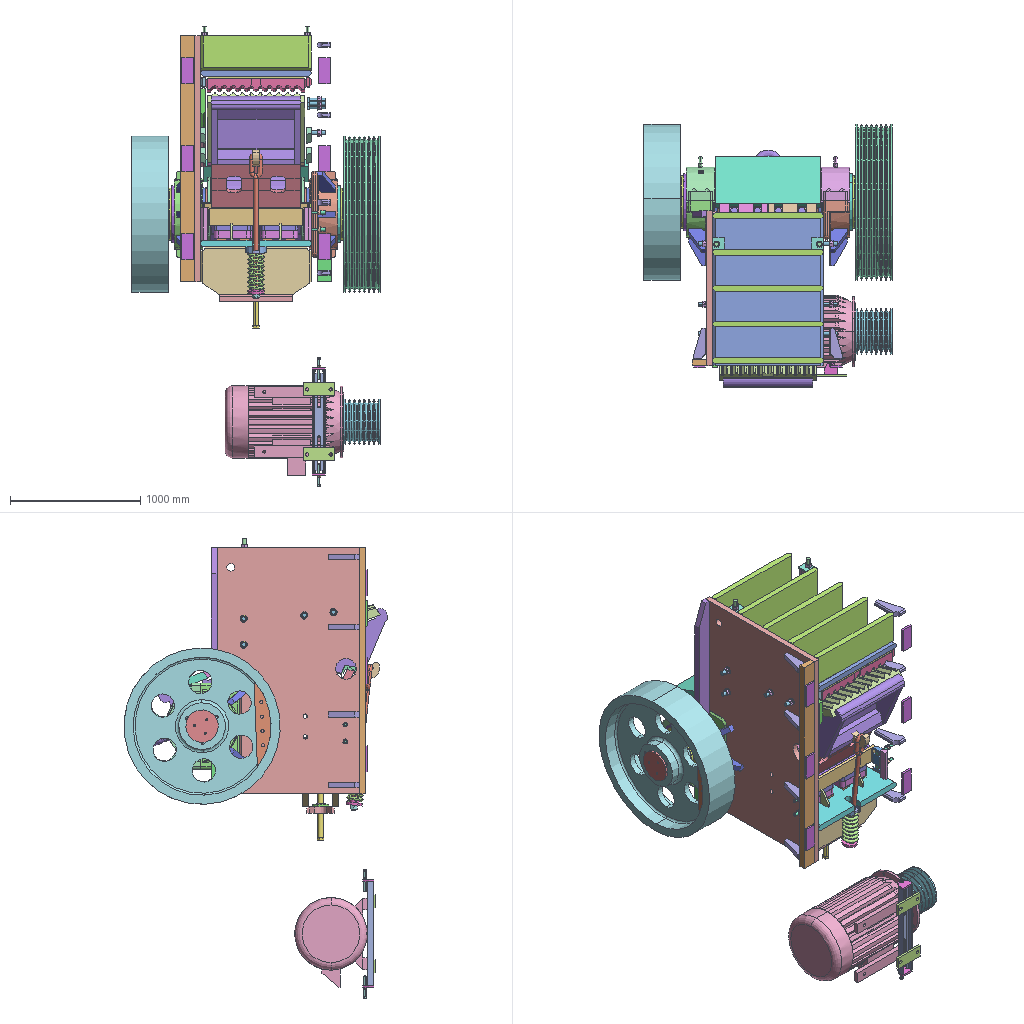Assembly | SolidWorks | 99 different items | 206 placed | box 1906 x 2026 x 3532 mm
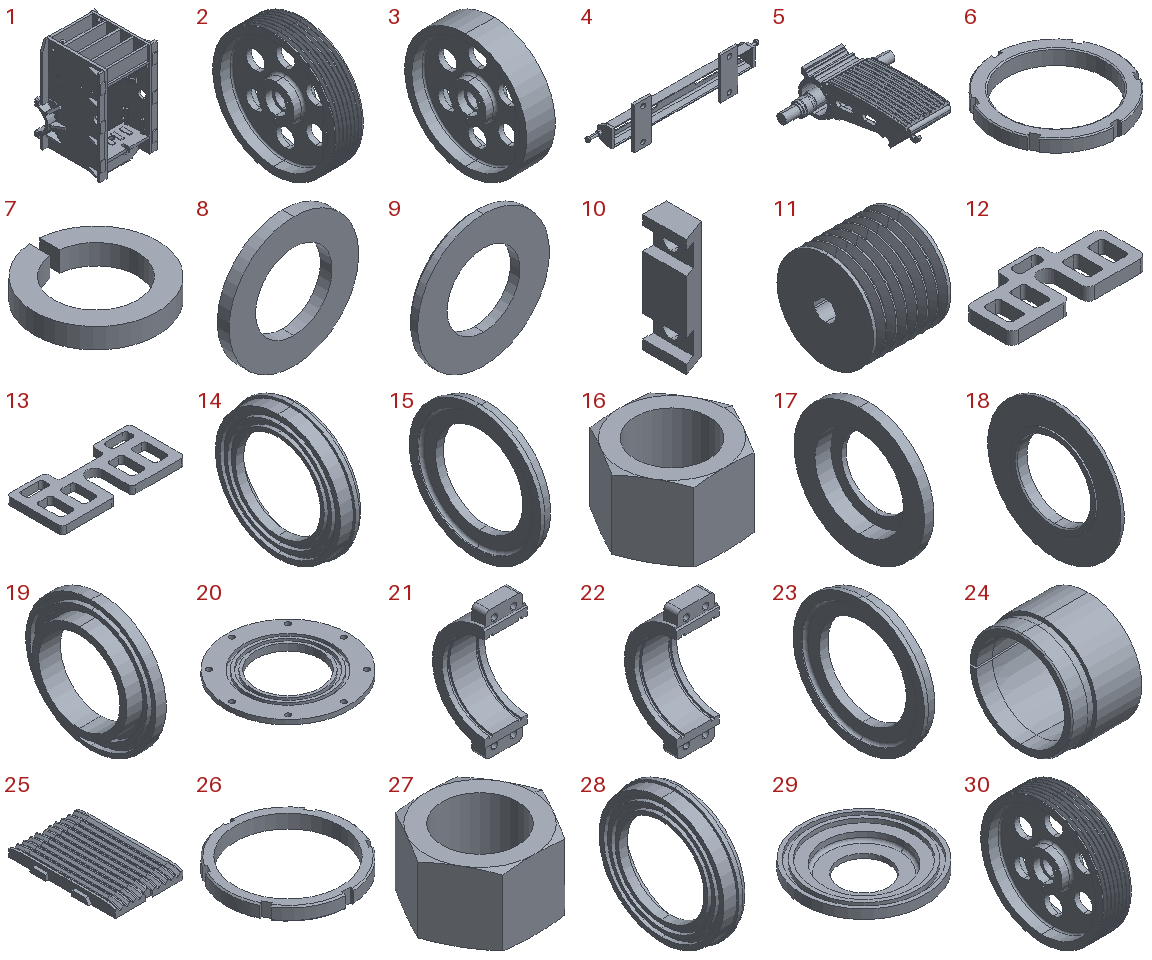Parts list (item | name | quantity | parent item | size | volume | features):
1 | (subassembly) | x1 | - | 1256 x 1280 x 2040 mm | 426098294 mm3 | features ReferencePattern 27, MirrorCompFeat 8, LocalCirPattern 2, LocalLPattern 1
2 | (subassembly) | x1 | - | 280 x 1200 x 1200 mm | 105552059 mm3 | features CompositeCurve 1
3 | (subassembly) | x1 | - | 280 x 1200 x 1200 mm | 122097534 mm3 | -
4 | (subassembly) | x1 | - | 984.816 x 100 x 240 mm | 1918082 mm3 | features ReferencePattern 4, MirrorCompFeat 3
5 | (subassembly) | x1 | - | 1846 x 2050 x 710.858 mm | 325009272 mm3 | features CompositeCurve 1
6 | - | x2 | - | 240 x 239.437 x 30 mm | 460595 mm3 | features Chamfer 3, CirPattern 1, Cut 1, Extrusion 1
7 | - | x4 | in 2 | 36.439 x 36.377 x 6 mm | 3321 mm3 | features Extrusion 1
8 | - | x4 | in 2 | 44 x 4 x 44 mm | 3958 mm3 | features Revolution 1
9 | - | x8 | - | 56 x 4 x 56 mm | 6746 mm3 | features Revolution 1
10 | - | x2 | - | 40 x 74.559 x 200 mm | 417359 mm3 | features ICE 2, Extrusion 1, MirrorPattern 1
11 | - | x1 | - | 280 x 349 x 349 mm | 15090387 mm3 | features ICE 1, LPattern 1, RevCut 1, Revolution 1
12 | - | x1 | - | 640 x 290 x 60 mm | 5683176 mm3 | features Fillet 2, Extrusion 1, ICE 1, MirrorPattern 1, PLine 1
13 | - | x1 | - | 640 x 290 x 40 mm | 4114262 mm3 | features Fillet 2, Extrusion 1, ICE 1, MirrorPattern 1, PLine 1
14 | - | x1 | - | 71 x 455 x 455 mm | 3180516 mm3 | features Revolution 1
15 | - | x1 | - | 41 x 455 x 455 mm | 2264387 mm3 | features Fillet 1, Revolution 1
16 | - | x2 | in 4 | 26.17 x 22.664 x 15.9 mm | 3864 mm3 | features Cut 2, Chamfer 1, Extrusion 1
17 | - | x2 | - | 63 x 404 x 404 mm | 2394632 mm3 | features Revolution 1
18 | - | x2 | - | 35 x 436 x 436 mm | 1356536 mm3 | features Chamfer 1, Revolution 1
19 | - | x2 | - | 64 x 384 x 384 mm | 2278534 mm3 | features Revolution 1
20 | - | x2 | - | 540 x 540 x 45 mm | 4136152 mm3 | features CirPattern 1, ICE 1, Revolution 1
21 | - | x1 | - | 218 x 352.5 x 660 mm | 9674169 mm3 | features ICE 5, 3DProfileFeature 1, Extrusion 1, Fillet 1, HoleWzd 1, MirrorPattern 1, RevCut 1, Revolution 1
22 | - | x1 | - | 218 x 352.5 x 660 mm | 9674169 mm3 | features ICE 5, 3DProfileFeature 1, Extrusion 1, Fillet 1, HoleWzd 1, MirrorPattern 1, RevCut 1, Revolution 1
23 | - | x1 | - | 44 x 455 x 455 mm | 2505652 mm3 | features Fillet 1, Revolution 1
24 | - | x2 | - | 151 x 239.983 x 240 mm | 1801757 mm3 | features Chamfer 1, ICE 1, Revolution 1
25 | - | x1 | - | 820 x 1170 x 110 mm | 61269041 mm3 | features Fillet 3, ICE 3, LPattern 3, MirrorPattern 2, Extrusion 1, SweepCut 1
26 | - | x2 | - | 270 x 269.399 x 30 mm | 439038 mm3 | features Chamfer 1, CirPattern 1, ICE 1, Revolution 1
27 | - | x4 | - | 39.55 x 34.251 x 22.3 mm | 12527 mm3 | features Cut 2, Chamfer 1, Extrusion 1
28 | - | x1 | - | 74 x 455 x 455 mm | 3257613 mm3 | features Revolution 1
29 | - | x2 | - | 404 x 404 x 56 mm | 2436851 mm3 | features Fillet 1, Revolution 1
30 | - | x1 | in 2 | 280 x 1200 x 1200 mm | 100101767 mm3 | features CirPattern 2, ICE 2, 3DProfileFeature 1, HoleWzd 1, LPattern 1, RevCut 1, Revolution 1
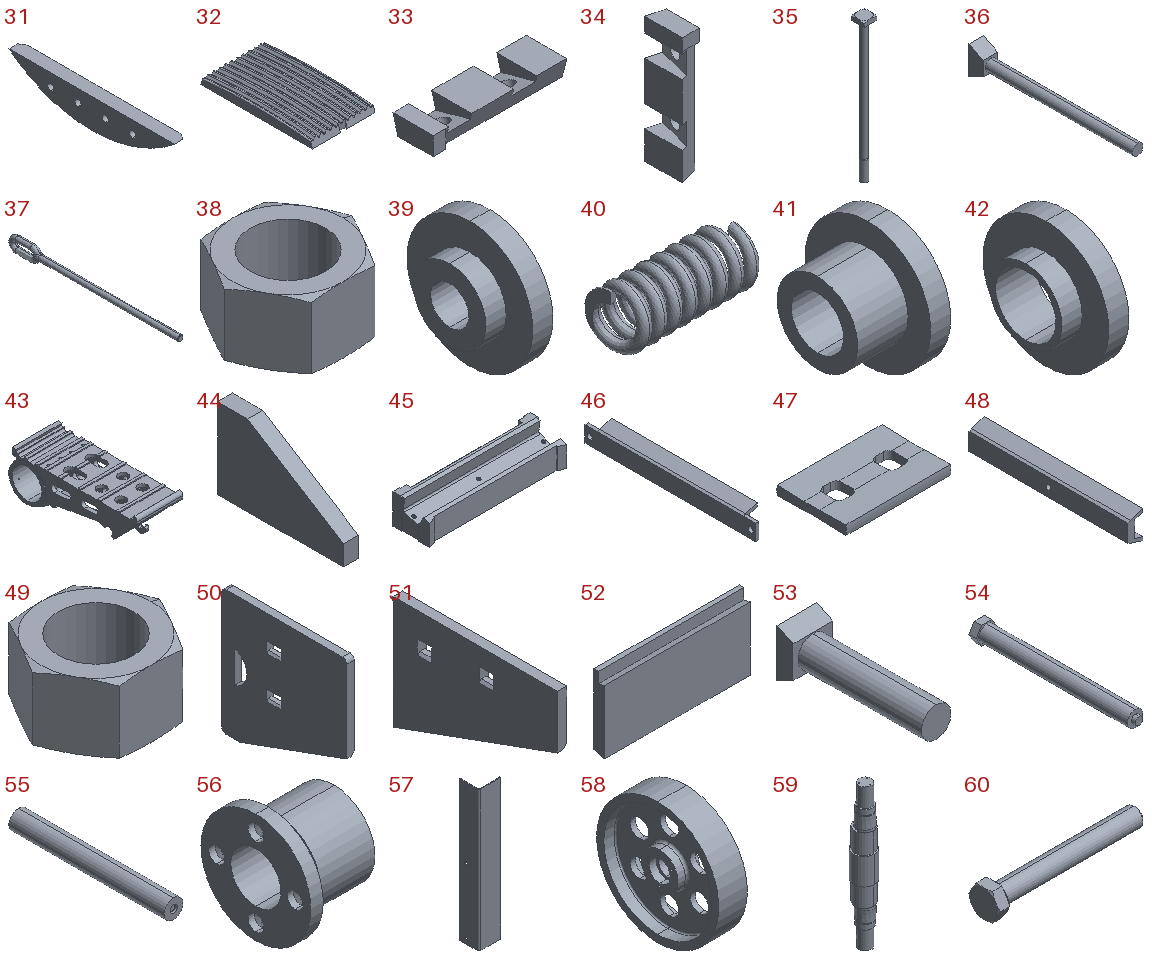31 | - | x4 | in 2, 3 | 50 x 666.801 x 118 mm | 2510197 mm3 | features Chamfer 1, Extrusion 1, ICE 1
32 | - | x1 | - | 750 x 1330 x 125.858 mm | 65171136 mm3 | features ICE 4, LPattern 2, MirrorPattern 2, Extrusion 1, Fillet 1, SweepCut 1
33 | - | x1 | - | 370 x 110.795 x 50 mm | 1371734 mm3 | features ICE 3, Extrusion 1, LPattern 1, RevCut 1
34 | - | x1 | - | 50 x 110.795 x 370 mm | 1371734 mm3 | features ICE 3, Extrusion 1, LPattern 1, RevCut 1
35 | - | x4 | - | 55 x 55 x 609 mm | 405608 mm3 | features Cut 1, Extrusion 1, Fillet 1, LPattern 1, RevCut 1, Revolution 1
36 | - | x2 | - | 40 x 450 x 80 mm | 385812 mm3 | features ICE 2, Extrusion 1
37 | - | x1 | - | 36 x 1131 x 102 mm | 1361962 mm3 | features Chamfer 1, Sweep 1
38 | - | x10 | - | 50.85 x 44.037 x 26.4 mm | 25591 mm3 | features Cut 2, Chamfer 1, Extrusion 1
39 | - | x1 | - | 40 x 125 x 125 mm | 281502 mm3 | features Revolution 1
40 | - | x1 | - | 280.817 x 125 x 125 mm | 1207735 mm3 | features Helix 1, ICE 1, Sweep 1
41 | - | x1 | - | 70 x 125 x 125 mm | 348104 mm3 | features Revolution 1
42 | - | x1 | - | 40 x 125 x 125 mm | 213770 mm3 | features Revolution 1
43 | - | x1 | - | 704 x 2050 x 634.865 mm | 188123623 mm3 | features ICE 12, MirrorPattern 5, 3DProfileFeature 4, HoleWzd 4, Fillet 2, CirPattern 1, Extrusion 1, Revolution 1
44 | - | x2 | - | 15 x 125 x 80 mm | 107250 mm3 | features Extrusion 1
45 | - | x1 | - | 800 x 215 x 175 mm | 15797212 mm3 | features ICE 5, 3DProfileFeature 2, HoleWzd 2, Extrusion 1, Fillet 1, MirrorPattern 1
46 | - | x1 | - | 65 x 800 x 120 mm | 2622134 mm3 | features ICE 2, Extrusion 1, MirrorPattern 1
47 | - | x1 | - | 680 x 450 x 60 mm | 14870230 mm3 | features Extrusion 1, ICE 1, MirrorPattern 1
48 | - | x1 | - | 65 x 682 x 120 mm | 2487309 mm3 | features Extrusion 1, ICE 1
49 | - | x1 | - | 60.79 x 52.646 x 31.9 mm | 43950 mm3 | features Cut 2, Chamfer 1, Extrusion 1
50 | - | x2 | - | 35 x 600 x 600 mm | 10412431 mm3 | features Chamfer 1, Extrusion 1, Fillet 1, ICE 1
51 | - | x2 | - | 35 x 600 x 413 mm | 6164844 mm3 | features ICE 2, Chamfer 1, Extrusion 1
52 | - | x1 | - | 800 x 60 x 400 mm | 17282858 mm3 | features Extrusion 1
53 | - | x8 | - | 40 x 140 x 48 mm | 113250 mm3 | features ICE 2, Extrusion 1
54 | - | x1 | - | 53 x 410 x 45.899 mm | 516586 mm3 | features ICE 1, Revolution 1
55 | - | x1 | - | 48 x 395 x 48 mm | 696230 mm3 | features 3DProfileFeature 1, HoleWzd 1, Revolution 1
56 | - | x1 | - | 50 x 70 x 70 mm | 75479 mm3 | features 3DProfileFeature 1, CirPattern 1, HoleWzd 1, Revolution 1
57 | - | x1 | - | 100 x 90 x 645 mm | 355061 mm3 | features FlatPattern 1, ICE 1, SMBaseFlange 1, SheetMetal 1
58 | - | x1 | in 3 | 280 x 1200 x 1200 mm | 117077142 mm3 | features CirPattern 2, ICE 2, 3DProfileFeature 1, HoleWzd 1, Revolution 1
59 | - | x1 | - | 270 x 270 x 1846 mm | 68110959 mm3 | features MirrorPattern 3, Revolution 2, 3DProfileFeature 1, CirPattern 1, HoleWzd 1, ICE 1
60 | - | x4 | in 2 | 200 x 41.569 x 36 mm | 100195 mm3 | features RevCut 4, Chamfer 1, Extrusion 1, Fillet 1, LPattern 1, Revolution 1
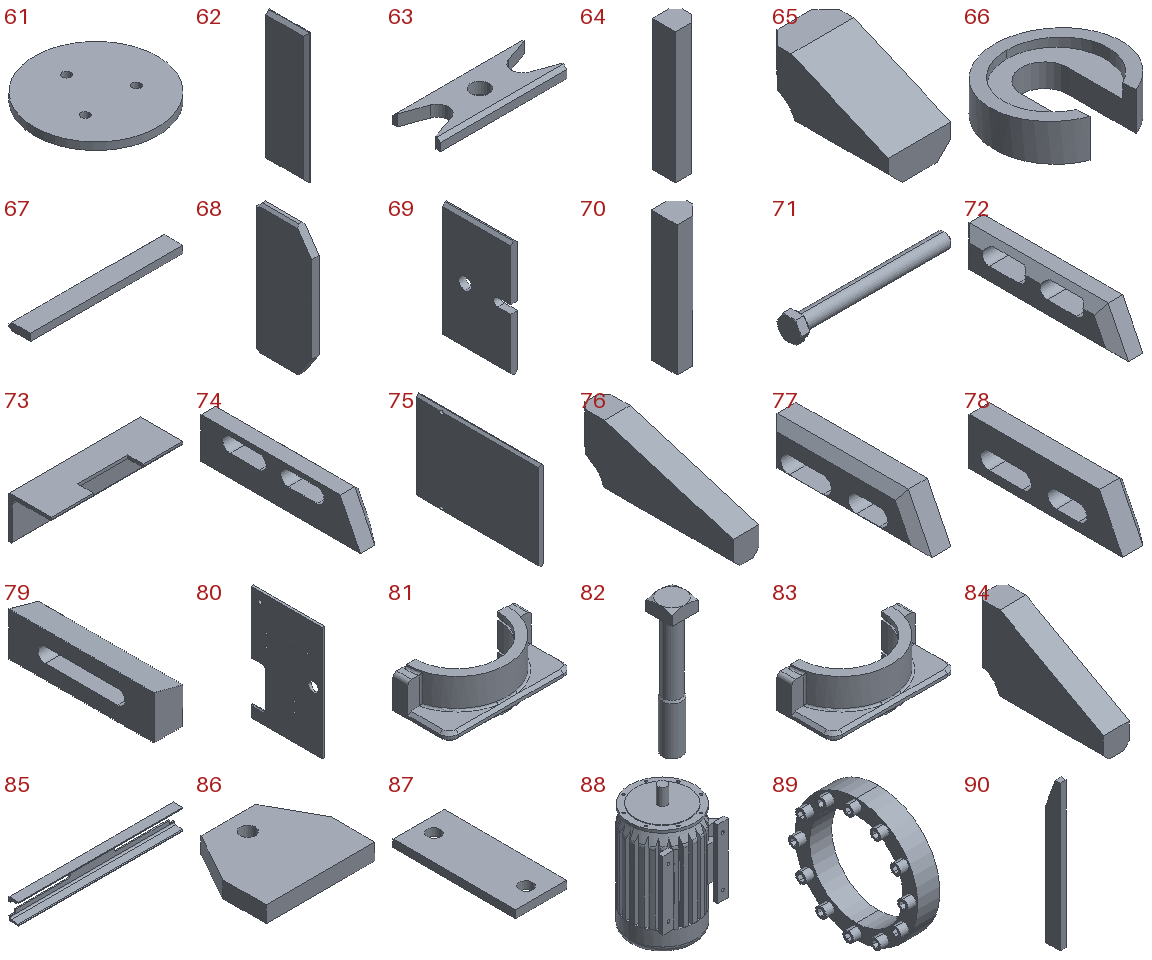61 | - | x2 | - | 250 x 250 x 15 mm | 726097 mm3 | features Extrusion 1
62 | - | x5 | in 1 | 45 x 265 x 850 mm | 9594917 mm3 | features Chamfer 1, Extrusion 1
63 | - | x1 | in 1 | 560 x 210 x 50 mm | 3864002 mm3 | features Chamfer 1, Extrusion 1
64 | - | x2 | in 1 | 50 x 50 x 280 mm | 637000 mm3 | features Chamfer 1, Extrusion 1
65 | - | x4 | in 1 | 45 x 90 x 50 mm | 124093 mm3 | features Chamfer 1, Extrusion 1
66 | - | x1 | in 1 | 160 x 154.162 x 49.592 mm | 478394 mm3 | features ICE 2, Revolution 1
67 | - | x2 | in 1 | 850 x 120 x 40 mm | 3888750 mm3 | features Chamfer 1, Extrusion 1
68 | - | x2 | in 1 | 50 x 370 x 850 mm | 14620496 mm3 | features Chamfer 1, Extrusion 1
69 | - | x1 | in 1 | 50 x 500 x 850 mm | 20176228 mm3 | features Chamfer 1, Extrusion 1
70 | - | x2 | in 1 | 50 x 50 x 250 mm | 525000 mm3 | features Chamfer 1, Extrusion 1
71 | - | x2 | in 4 | 170 x 27.713 x 24 mm | 37050 mm3 | features RevCut 4, Chamfer 1, Extrusion 1, Fillet 1, LPattern 1, Revolution 1
72 | - | x1 | in 1 | 40 x 275 x 70 mm | 515457 mm3 | features Chamfer 1, Extrusion 1
73 | - | x2 | in 1 | 250 x 80 x 80 mm | 217898 mm3 | features ICE 1, WeldMemberFeat 1, WeldmentFeature 1
74 | - | x1 | in 1 | 40 x 275 x 70 mm | 515457 mm3 | features Chamfer 1, Extrusion 1
75 | - | x1 | in 1 | 45 x 1170 x 850 mm | 43736327 mm3 | features Chamfer 1, Extrusion 1
76 | - | x8 | in 1 | 40 x 240 x 100 mm | 643693 mm3 | features Chamfer 1, Extrusion 1
77 | - | x1 | in 1 | 40 x 229 x 70 mm | 431150 mm3 | features Chamfer 1, Extrusion 1
78 | - | x1 | in 1 | 40 x 229 x 70 mm | 442689 mm3 | features Chamfer 1, Extrusion 1
79 | - | x4 | in 1 | 40 x 200 x 60 mm | 344562 mm3 | features Extrusion 1, ICE 1
80 | - | x2 | in 1 | 45 x 1185 x 1890 mm | 92721344 mm3 | features ICE 2, Chamfer 1, Extrusion 1, Fillet 1
81 | - | x1 | in 1 | 660 x 300 x 218 mm | 12799321 mm3 | features Fillet 3, ICE 2, MirrorPattern 2, 3DProfileFeature 1, Chamfer 1, Extrusion 1, HoleWzd 1, RevCut 1
82 | - | x4 | - | 32.173 x 32.173 x 165 mm | 73641 mm3 | features Cut 1, Extrusion 1, Fillet 1, LPattern 1, RevCut 1, Revolution 1
83 | - | x1 | in 1 | 660 x 300 x 218 mm | 12799321 mm3 | features Fillet 3, ICE 2, MirrorPattern 2, 3DProfileFeature 1, Chamfer 1, Extrusion 1, HoleWzd 1, RevCut 1
84 | - | x6 | in 1 | 45 x 220 x 140 mm | 896409 mm3 | features Chamfer 1, Extrusion 1
85 | - | x1 | in 4 | 800 x 48 x 100 mm | 931477 mm3 | features ICE 2, MirrorPattern 1, WeldMemberFeat 1, WeldmentFeature 1
86 | - | x2 | in 4 | 100 x 85 x 15 mm | 108316 mm3 | features 3DProfileFeature 1, Extrusion 1, HoleWzd 1
87 | - | x2 | in 4 | 100 x 240 x 15 mm | 344072 mm3 | features Extrusion 1, ICE 1
88 | - | x1 | - | 687.6 x 557.6 x 1050 mm | 215841244 mm3 | features Boss 7, Cut 3, CirPattern 2, Chamfer 1, Extrusion 1, Fillet 1
89 | - | x2 | - | 52 x 210 x 210 mm | 580630 mm3 | features CirPattern 1, ICE 1, Revolution 1
90 | - | x2 | in 1 | 45 x 110 x 1110 mm | 5170500 mm3 | features Extrusion 1
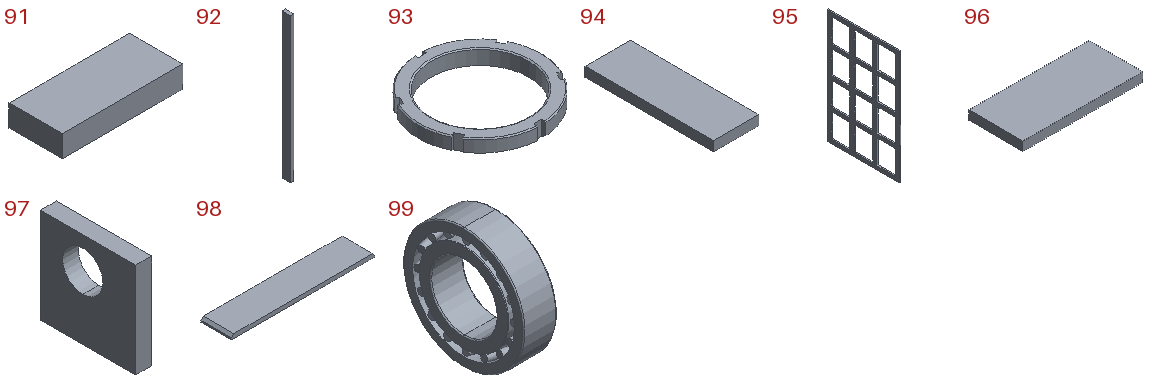91 | - | x2 | in 1 | 250 x 110 x 45 mm | 1237500 mm3 | features Extrusion 1
92 | - | x2 | in 1 | 45 x 110 x 1890 mm | 9355500 mm3 | features Extrusion 1
93 | - | x2 | - | 240 x 239.437 x 30 mm | 460595 mm3 | features Chamfer 3, CirPattern 1, Cut 1, Extrusion 1
94 | - | x4 | in 1 | 70 x 200 x 15 mm | 210000 mm3 | features Extrusion 1
95 | - | x1 | in 1 | 15 x 740 x 1170 mm | 4693500 mm3 | features Extrusion 1, ICE 1, MirrorPattern 1
96 | - | x6 | in 1 | 200 x 90 x 15 mm | 270000 mm3 | features Extrusion 1
97 | - | x2 | in 1 | 15 x 90 x 90 mm | 104488 mm3 | features Extrusion 1, ICE 1
98 | - | x1 | in 1 | 850 x 180 x 40 mm | 5852250 mm3 | features Chamfer 1, Extrusion 1
99 | - | x4 | - | 120 x 440 x 440 mm | 10049634 mm3 | features Revolution 3, CirPattern 1, MirrorPattern 1
Mates (type | each side: item.copy, entity, surface, feature):
In the top assembly
Coincident | 81.1 plane | assembly plane
Coincident | 1.1 plane | assembly plane | 2 times
Coincident | 95.1 face plane Boss-Extrude1 | 25.1 face plane Boss-Extrude1
Coincident | 25.1 plane | assembly plane
Coincident | 62.1 face plane Boss-Extrude1 | 25.1 face plane Boss-Extrude1
Coincident | 59.1 plane | assembly plane
Concentric | 81.1 face cylinder Boss-Extrude1 | 59.1 face cone Revolve2
Concentric | 59.1 face cylinder Revolve1 | 18.1 face cylinder Revolve1
Coincident | 59.1 face plane Revolve1 | 18.1 face plane Revolve1
Concentric | 59.1 face cylinder Revolve1 | 99.1 face cylinder Boss-Revolve1
Coincident | 18.1 face plane Revolve1 | 99.1 face plane Boss-Revolve1
Concentric | 59.1 face cylinder Revolve1 | 20.1 face cylinder Revolve1
Coincident | 99.1 face plane Base-Revolve1 | 20.1 face plane Revolve1
Concentric | 59.1 face cylinder Revolve1 | 19.1 face cylinder Revolve1
Coincident | 99.1 face plane Boss-Revolve1 | 19.1 face plane Revolve1
Coincident | 19.1 face plane Revolve1 | 17.1 face plane Revolve1
Concentric | 59.1 face cylinder Revolve2 | 17.1 face cylinder Revolve1
Concentric | 81.1 face cylinder Boss-Extrude1 | 23.1 face cylinder Revolve1
Coincident | 81.1 face plane Cut-Revolve1 | 23.1 face plane Revolve1
Concentric | 59.1 face cylinder Revolve2 | 24.1 face cylinder Revolve1
Coincident | 17.1 face plane Revolve1 | 24.1 face plane Revolve1
Concentric | 59.1 face cylinder Revolve2 | 28.1 face cylinder Revolve1
Coincident | 43.1 plane | assembly plane
Concentric | 59.1 face cylinder Revolve1 | 43.1 face cylinder Boss-Extrude1
Concentric | 20.1 face cylinder Cut-Extrude1 | 43.1 face cylinder CirPattern1
Coincident | 81.1 face plane Cut-Revolve1 | 28.1 face plane Revolve1
Concentric | 59.1 face cylinder Revolve2 | 99.2 face cylinder Base-Revolve1
Coincident | 23.1 face plane Revolve1 | 99.2 face plane Base-Revolve1
Concentric | 59.1 face cylinder Revolve2 | 26.1 face cylinder Revolve1
Coincident | 99.2 face plane Boss-Revolve1 | 26.1 face plane Revolve1
Concentric | 59.1 face cylinder Revolve2 | 93.1 face cylinder Base-Extrude
Concentric | 59.1 face cylinder Revolve2 | 6.1 face cylinder Base-Extrude
Coincident | 93.1 face plane Base-Extrude | 6.1 face plane Base-Extrude
Coincident | 26.1 face plane Revolve1 | 93.1 face plane Base-Extrude
Concentric | 59.1 face cylinder Revolve2 | 29.1 face cylinder Revolve1
Coincident | 59.1 face plane Revolve2 | 29.1 face plane Revolve1
Concentric | 81.1 face cylinder M30 Tapped Hole2 | 21.1 face cylinder Mirror1 | 2 times
Coincident | 81.1 face plane Boss-Extrude1 | 21.1 face plane Boss-Extrude2
Concentric | 59.1 face cylinder Revolve2 | 30.1 face cylinder Revolve1
Coincident | 29.1 face plane Revolve1 | 30.1 face plane Revolve1
Concentric | 59.1 face cylinder Revolve2 | 58.1 face cylinder Revolve1
Concentric | 59.1 face cylinder Mirror1 | 24.2 face cylinder Revolve1
Coincident | 17.2 face plane Revolve1 | 24.2 face plane Revolve1
Concentric | 59.1 face cylinder Mirror1 | 26.2 face cylinder Revolve1
Concentric | 59.1 face cylinder Mirror1 | 6.2 face cylinder Base-Extrude
Concentric | 59.1 face cylinder Mirror1 | 93.2 face cylinder Base-Extrude
Concentric | 59.1 face cylinder Mirror1 | 15.1 face cylinder Revolve1
Concentric | 59.1 face cylinder Mirror1 | 14.1 face cylinder Revolve1
Concentric | 59.1 face cylinder Mirror1 | 22.1 face cylinder Boss-Extrude2
Concentric | 83.1 face cylinder M30 Tapped Hole2 | 22.1 face cylinder Cut-Extrude1
Parallel | 80.1 face plane Boss-Extrude1 | 22.1 face plane Boss-Extrude3
Concentric | 59.1 face cylinder Mirror1 | 99.3 face cylinder Base-Revolve1
Coincident | 83.1 face plane Cut-Revolve1 | 14.1 face plane Revolve1
Coincident | 83.1 face plane Cut-Revolve1 | 15.1 face plane Revolve1
DistanceDim | 99.3 face plane Base-Revolve1 | 14.1 face plane Revolve1
Coincident | 26.2 face plane Revolve1 | 99.3 face plane Boss-Revolve1
Coincident | 93.2 face plane Base-Extrude | 6.2 face plane Base-Extrude
Coincident | 26.2 face plane Revolve1 | 93.2 face plane Base-Extrude
Concentric | 59.1 face cylinder Mirror1 | 29.2 face cylinder Revolve1
Coincident | 59.1 face plane Mirror1 | 29.2 face plane Revolve1
Coincident | 58.1 face plane Revolve1 | 29.2 face plane Revolve1
Concentric | 59.1 edge | 61.1 face cylinder Boss-Extrude1
Concentric | 59.1 edge | 89.1 face cylinder Revolve1
Coincident | 30.1 face plane Revolve1 | 89.1 face plane Revolve1
Coincident | 30.1 face plane Revolve1 | 61.1 face plane Boss-Extrude1
Concentric | 59.1 face cylinder M16 Tapped Hole1 | 61.1 face cylinder Boss-Extrude1
Coincident | 32.1 plane | assembly plane
Coincident | 43.1 face plane Boss-Extrude1 | 32.1 face plane Boss-Extrude1
Coincident | 43.1 face plane Boss-Extrude1 | 32.1 vertex
Coincident | 52.1 plane | assembly plane
Coincident | 43.1 face plane Boss-Extrude1 | 52.1 face plane Boss-Extrude1
Coincident | 43.1 face plane Boss-Extrude1 | 52.1 vertex
Concentric | 43.1 face cylinder Cut-Extrude2 | 34.1 face cylinder LPattern1
Concentric | 43.1 face cylinder Cut-Extrude2 | 34.1 face cylinder Cut-Revolve1
Coincident | 32.1 face plane Boss-Extrude1 | 34.1 vertex
Concentric | 43.1 face cylinder Cut-Extrude2 | 33.1 face cylinder LPattern1
Concentric | 43.1 face cylinder Cut-Extrude2 | 33.1 face cylinder Cut-Revolve1
Coincident | 32.1 face plane Boss-Extrude1 | 33.1 vertex
Concentric | 34.1 face cylinder Cut-Revolve1 | 35.1 face cylinder Boss-Revolve1
Coincident | 34.1 face plane Cut-Extrude2 | 35.1 vertex
Concentric | 33.1 face cylinder Cut-Revolve1 | 35.2 face cylinder Boss-Revolve1
Coincident | 33.1 face plane Cut-Extrude1 | 35.2 vertex
Coincident | 80.1 face plane Boss-Extrude1 | 51.1 face plane Boss-Extrude1
Parallel | 79.1 face plane Boss-Extrude1 | 51.1 face plane Boss-Extrude1
DistanceDim | 51.1 face plane Boss-Extrude1 | 80.1 face plane Boss-Extrude1
Tangent | 80.1 face cylinder Cut-Extrude1 | 51.1 face plane Cut-Extrude1
Coincident | 80.1 face plane Boss-Extrude1 | 50.1 face plane Boss-Extrude1
Parallel | 79.2 face plane Boss-Extrude1 | 50.1 face plane Boss-Extrude1
Tangent | 80.1 face cylinder Cut-Extrude1 | 50.1 face plane Cut-Extrude1
Coincident | 51.1 face plane Boss-Extrude1 | 50.1 face plane Boss-Extrude1
Concentric | 80.1 face cylinder Cut-Extrude1 | 53.1 face cylinder Boss-Extrude2
Concentric | 80.1 face cylinder Cut-Extrude1 | 53.2 face cylinder Boss-Extrude2
Concentric | 80.1 face cylinder Cut-Extrude1 | 53.3 face cylinder Boss-Extrude2
Concentric | 80.1 face cylinder Cut-Extrude1 | 53.4 face cylinder Boss-Extrude2
Coincident | 50.1 face plane Cut-Extrude1 | 53.2 edge
Coincident | 50.1 face plane Cut-Extrude1 | 53.1 edge
Coincident | 51.1 face plane Cut-Extrude1 | 53.3 edge
Coincident | 51.1 face plane Cut-Extrude2 | 53.4 edge
Concentric | 80.1 face cylinder Cut-Extrude1 | 9.1 face cylinder Base-Revolve
Coincident | 80.1 face plane Boss-Extrude1 | 9.1 face plane Base-Revolve
Concentric | 80.1 face cylinder Cut-Extrude1 | 9.2 face cylinder Base-Revolve
Coincident | 80.1 face plane Boss-Extrude1 | 9.2 face plane Base-Revolve
Concentric | 80.1 face cylinder Cut-Extrude1 | 9.3 face cylinder Base-Revolve
Coincident | 80.1 face plane Boss-Extrude1 | 9.3 face plane Base-Revolve
Concentric | 80.1 face cylinder Cut-Extrude1 | 9.4 face cylinder Base-Revolve
Coincident | 80.1 face plane Boss-Extrude1 | 9.4 face plane Base-Revolve
Concentric | 9.1 face cylinder Base-Revolve | 38.1 face cylinder Base-Extrude
Coincident | 9.1 face plane Base-Revolve | 38.1 face plane Base-Extrude
Concentric | 9.2 face cone Base-Revolve | 38.2 face cylinder Base-Extrude
Coincident | 9.2 face plane Base-Revolve | 38.2 face plane Base-Extrude
Concentric | 9.3 face cylinder Base-Revolve | 38.3 face cylinder Base-Extrude
Coincident | 9.3 face plane Base-Revolve | 38.3 face plane Base-Extrude
Concentric | 9.4 face cylinder Base-Revolve | 38.4 face cylinder Base-Extrude
Coincident | 9.4 face plane Base-Revolve | 38.4 face plane Base-Extrude
Symmetric | 43.1 face plane Boss-Extrude1 | 43.1 face plane Boss-Extrude1 | 48.1 plane
Concentric | 43.1 face cylinder M20 Tapped Hole1 | 48.1 face cylinder Cut-Extrude1
Coincident | 43.1 face plane Boss-Extrude1 | 48.1 face plane Boss-Extrude1
Coincident | 37.1 plane | assembly plane
Concentric | 43.1 edge | 37.1 select_type:24
DistanceDim | 32.1 vertex | 75.1 face plane Boss-Extrude1
PlanarAngleDim | 37.1 plane | 69.1 face plane Boss-Extrude1
Concentric | 66.1 face cylinder Revolve2 | 39.1 face cylinder Revolve1
Coincident | 66.1 face plane Revolve2 | 39.1 face plane Revolve1
Concentric | 39.1 face cylinder Revolve1 | 40.1 select_type:24
Coincident | 39.1 face plane Revolve1 | 40.1 face plane Cut-Extrude1
Concentric | 37.1 edge | 42.1 face cylinder Revolve1
Coincident | 40.1 vertex | 42.1 face plane Revolve1
Concentric | 42.1 edge | 49.1 edge
Coincident | 42.1 face plane Revolve1 | 49.1 face plane Base-Extrude
Coincident | 45.1 plane | assembly plane
Coincident | 46.1 plane | assembly plane
Symmetric | 45.1 face plane Boss-Extrude1 | 45.1 face plane Boss-Extrude1 | 46.1 plane
Coincident | 45.1 face plane Boss-Extrude1 | 46.1 face plane Boss-Extrude1
Concentric | 75.1 face cylinder Boss-Extrude1 | 36.1 face cylinder Boss-Extrude2
Coincident | 25.1 face plane Boss-Extrude2 | 36.1 edge
Concentric | 36.1 face cylinder Boss-Extrude2 | 38.5 face cylinder Base-Extrude
Coincident | 97.1 face plane Boss-Extrude1 | 38.5 face plane Base-Extrude
Coincident | 47.1 plane | assembly plane
Coincident | 70.1 face plane Boss-Extrude1 | 10.1 face plane Boss-Extrude1
DistanceDim | 10.1 face plane Boss-Extrude1 | 70.2 face plane Boss-Extrude1 | 2 times
Coincident | 45.1 face plane Cut-Extrude3 | 10.1 edge
Coincident | 12.1 plane | assembly plane
Coincident | 94.1 face plane Boss-Extrude1 | 12.1 face plane Boss-Extrude1
Coincident | 69.1 face plane Boss-Extrude1 | 44.1 face plane Boss-Extrude1
DistanceDim | assembly plane | 44.1 face plane Boss-Extrude1
Concentric | 10.1 face cylinder Cut-Extrude2 | 82.1 face cylinder Boss-Revolve1
Coincident | 10.1 face plane Mirror1 | 82.1 face plane Base-Extrude
Concentric | 10.1 face cylinder Cut-Extrude2 | 82.2 face cylinder Boss-Revolve1
Coincident | 10.1 face plane Cut-Extrude1 | 82.2 face plane Base-Extrude
Concentric | 82.1 face cone Cut-Revolve1 | 27.1 face cylinder Base-Extrude
Concentric | 82.2 face cone Cut-Revolve1 | 27.2 face cylinder Base-Extrude
Coincident | 80.1 face plane Boss-Extrude1 | 27.1 face plane Base-Extrude
Coincident | 80.1 face plane Boss-Extrude1 | 27.2 face plane Base-Extrude
Coincident | 94.2 face plane Boss-Extrude1 | 44.1 face plane Boss-Extrude1
Coincident | 44.1 face plane Boss-Extrude1 | 12.1 face plane Boss-Extrude1
Coincident | 13.1 plane | assembly plane
Coincident | 12.1 face plane Boss-Extrude1 | 13.1 face plane Boss-Extrude1
Coincident | 44.1 face plane Boss-Extrude1 | 13.1 face plane Boss-Extrude1
Coincident | 45.1 face plane Boss-Extrude1 | 13.1 face plane Boss-Extrude1
PlanarAngleDim | 47.1 face plane Boss-Extrude1 | 96.1 face plane Boss-Extrude1
Tangent | 46.1 face plane Boss-Extrude1 | 47.1 face cylinder Boss-Extrude1
Concentric | 63.1 edge | 41.1 face cylinder Revolve1
Coincident | 63.1 face plane Boss-Extrude1 | 41.1 face plane Revolve1
Coincident | 96.2 face plane Boss-Extrude1 | 88.1 face plane Extrude7
Concentric | 88.1 face cylinder Extrude1 | 11.1 face cylinder LPattern1
Coincident | 88.1 face plane Extrude2 | 11.1 face plane Revolve1
Coincident | 30.1 face plane Revolve1 | 11.1 face plane Revolve1
DistanceDim | 88.1 face plane Extrude7 | 92.1 face plane Boss-Extrude1
BeltDim | 30.1 face cylinder LPattern1 | 11.1 face cylinder LPattern1
Concentric | 41.1 face cylinder Revolve1 | 54.1 face cylinder Revolve1
Concentric | 54.1 face cylinder Revolve1 | 56.1 face cylinder Revolve1
Coincident | 41.1 face plane Revolve1 | 56.1 face plane Revolve1
Concentric | 54.1 face cylinder Revolve1 | 55.1 face cylinder Revolve1
Coincident | 54.1 face plane Revolve1 | 55.1 face plane Revolve1
Coincident | 57.1 plane | assembly plane
Concentric | 43.1 face cylinder Cut-Extrude5 | 57.1 face cylinder Cut-Extrude1
Coincident | 88.1 face plane Extrude7 | 85.1 face plane hot-rolled channel steel (GB/T 707-1988) 10(1)
Symmetric | 88.1 face plane Extrude7 | 88.1 face plane Extrude7 | 4.1 plane
DistanceDim | 85.1 face plane hot-rolled channel steel (GB/T 707-1988) 10(1) | 88.1 face plane Extrude7
In subassembly 1
Coincident | 80.2 face plane Boss-Extrude1 | 80.3 face plane Boss-Extrude1 | 2 times
DistanceDim | 80.2 face plane Boss-Extrude1 | 80.3 face plane Boss-Extrude1
Coincident | 80.2 face plane Boss-Extrude1 | 75.2 face plane Boss-Extrude1
Symmetric | 80.2 face plane Boss-Extrude1 | 80.3 face plane Boss-Extrude1 | 75.2 plane
DistanceDim | 75.2 face plane Boss-Extrude1 | 80.2 face plane Boss-Extrude1
Coincident | 80.2 plane | 1.2 plane | 2 times
Coincident | 75.2 plane | 1.2 plane
Coincident | 62.2 plane | 1.2 plane
Coincident | 75.2 face plane Boss-Extrude1 | 62.2 face plane Boss-Extrude1 | 2 times
Coincident | 62.3 plane | 1.2 plane
Coincident | 75.2 face plane Boss-Extrude1 | 62.3 face plane Boss-Extrude1
DistanceDim | 62.3 face plane Boss-Extrude1 | 62.2 face plane Boss-Extrude1
Coincident | 62.4 plane | 1.2 plane
DistanceDim | 62.4 face plane Boss-Extrude1 | 62.5 face plane Boss-Extrude1
Coincident | 75.2 face plane Boss-Extrude1 | 62.4 face plane Boss-Extrude1
Coincident | 62.3 face plane Boss-Extrude1 | 73.1 face plane hot-rolled equal angle steel (GB/T 9787-1988) 80×6(1)
Coincident | 75.2 face plane Boss-Extrude1 | 73.1 face plane hot-rolled equal angle steel (GB/T 9787-1988) 80×6(1)
DistanceDim | 73.1 face plane hot-rolled equal angle steel (GB/T 9787-1988) 80×6(1) | 80.2 face plane Boss-Extrude1
Concentric | 75.2 face cylinder Boss-Extrude1 | 97.2 face cylinder Cut-Extrude1
Coincident | 73.1 face plane hot-rolled equal angle steel (GB/T 9787-1988) 80×6(1) | 97.2 face plane Boss-Extrude1
Parallel | 80.2 face plane Boss-Extrude1 | 97.2 face plane Boss-Extrude1
Coincident | 80.2 face plane Boss-Extrude1 | 92.2 face plane Boss-Extrude1 | 3 times
Coincident | 80.3 face plane Boss-Extrude1 | 77.1 face plane Boss-Extrude1
Coincident | 75.2 face plane Boss-Extrude1 | 77.1 face plane Boss-Extrude1
Coincident | 80.2 face plane Boss-Extrude1 | 78.1 face plane Boss-Extrude1
Coincident | 75.2 face plane Boss-Extrude1 | 78.1 face plane Boss-Extrude1
Coincident | 80.3 face plane Boss-Extrude1 | 72.1 face plane Boss-Extrude1
DistanceDim | 72.1 face plane Boss-Extrude1 | 80.3 face plane Boss-Extrude1
Coincident | 80.2 face plane Boss-Extrude1 | 74.1 face plane Boss-Extrude1
Coincident | 78.1 face plane Boss-Extrude1 | 74.1 face plane Boss-Extrude1
Coincident | 72.1 face plane Boss-Extrude1 | 74.1 face plane Boss-Extrude1
DistanceDim | 77.1 face plane Boss-Extrude1 | 75.2 face plane Boss-Extrude1
DistanceDim | 78.1 face plane Boss-Extrude1 | 75.2 face plane Boss-Extrude1
Coincident | 77.1 face plane Boss-Extrude1 | 72.1 face plane Boss-Extrude1
Coincident | 95.2 plane | 1.2 plane
Coincident | 75.2 face plane Boss-Extrude1 | 95.2 face plane Boss-Extrude1 | 2 times
Coincident | 80.2 face plane Boss-Extrude1 | 96.3 face plane Boss-Extrude1
Symmetric | 92.2 plane | 96.3 face plane Boss-Extrude1 | 96.3 face plane Boss-Extrude1
DistanceDim | 96.3 face plane Boss-Extrude1 | 80.2 face plane Boss-Extrude1
Coincident | 92.2 face plane Boss-Extrude1 | 96.4 face plane Boss-Extrude1
Coincident | 96.3 face plane Boss-Extrude1 | 96.4 face plane Boss-Extrude1
Coincident | 92.2 face plane Boss-Extrude1 | 96.5 face plane Boss-Extrude1
Coincident | 96.3 face plane Boss-Extrude1 | 96.5 face plane Boss-Extrude1
DistanceDim | 96.4 face plane Boss-Extrude1 | 96.3 face plane Boss-Extrude1
DistanceDim | 96.5 face plane Boss-Extrude1 | 96.4 face plane Boss-Extrude1
Coincident | 80.3 face plane Boss-Extrude1 | 79.3 face plane Boss-Extrude1
PlanarAngleDim | 79.3 face plane Boss-Extrude1 | 75.2 face plane Boss-Extrude1
Coincident | 80.3 face plane Boss-Extrude1 | 79.4 face plane Boss-Extrude1
Coincident | 79.3 face plane Boss-Extrude1 | 79.4 face plane Boss-Extrude1
DistanceDim | 79.3 face plane Boss-Extrude1 | 79.4 face plane Boss-Extrude1
DistanceDim | 79.4 vertex | 80.3 face plane Boss-Extrude1
DistanceDim | 72.1 face plane Boss-Extrude1 | 79.4 vertex
Width | 80.3 face plane Boss-Extrude1 | 80.3 face plane Boss-Extrude1 | 81.2 face plane Cut-Extrude1 | 81.2 face plane Boss-Extrude2
Width | 80.3 face plane Boss-Extrude1 | 80.3 face plane Boss-Extrude1 | 81.2 face plane Boss-Extrude1 | 81.2 face plane Boss-Extrude1
Coincident | 80.3 face plane Boss-Extrude1 | 81.2 face plane Boss-Extrude2
Coincident | 80.2 face plane Boss-Extrude1 | 84.1 face plane Boss-Extrude1
Coincident | 81.2 plane | 84.1 plane
Coincident | 98.1 plane | 1.2 plane
DistanceDim | 98.1 face plane Boss-Extrude1 | 80.3 face plane Boss-Extrude1 | 2 times
Coincident | 67.1 plane | 1.2 plane
Coincident | 98.1 face plane Boss-Extrude1 | 67.1 face plane Boss-Extrude1 | 2 times
Coincident | 67.2 plane | 1.2 plane
Coincident | 98.1 face plane Boss-Extrude1 | 67.2 face plane Boss-Extrude1 | 2 times
Coincident | 69.2 plane | 1.2 plane
DistanceDim | 69.2 face plane Boss-Extrude1 | 80.3 face plane Boss-Extrude1
DistanceDim | 69.2 face plane Boss-Extrude1 | 96.3 face plane Boss-Extrude1
Coincident | 68.1 plane | 1.2 plane
DistanceDim | 69.2 face plane Boss-Extrude1 | 68.1 face plane Boss-Extrude1
Coincident | 69.2 face plane Boss-Extrude1 | 68.1 face plane Boss-Extrude1
Coincident | 68.2 plane | 1.2 plane
Coincident | 69.2 face plane Boss-Extrude1 | 68.2 face plane Boss-Extrude1
DistanceDim | 68.1 face plane Boss-Extrude1 | 68.2 face plane Boss-Extrude1
Coincident | 80.2 face plane Boss-Extrude1 | 90.1 face plane Boss-Extrude1 | 3 times
Coincident | 80.2 face plane Boss-Extrude1 | 91.1 face plane Boss-Extrude1 | 3 times
Coincident | 63.2 plane | 1.2 plane
Symmetric | 68.1 face plane Boss-Extrude1 | 68.2 face plane Boss-Extrude1 | 63.2 plane
Coincident | 68.1 face plane Boss-Extrude1 | 63.2 face plane Boss-Extrude1
Concentric | 69.2 face cylinder Boss-Extrude1 | 66.2 face cylinder Cut-Extrude2
Parallel | 80.2 face plane Boss-Extrude1 | 66.2 face plane Cut-Extrude2
Coincident | 69.2 face plane Boss-Extrude1 | 66.2 face plane Revolve2
Coincident | 80.3 face plane Boss-Extrude1 | 64.1 face plane Boss-Extrude1
Coincident | 69.2 face plane Boss-Extrude1 | 64.1 face plane Boss-Extrude1
DistanceDim | 64.1 face plane Boss-Extrude1 | 96.6 face plane Boss-Extrude1
Coincident | 80.3 face plane Boss-Extrude1 | 70.3 face plane Boss-Extrude1
Coincident | 69.2 face plane Boss-Extrude1 | 70.3 face plane Boss-Extrude1
DistanceDim | 64.1 face plane Boss-Extrude1 | 70.3 face plane Boss-Extrude1
Coincident | 64.1 face plane Boss-Extrude1 | 65.1 face plane Boss-Extrude1
Coincident | 80.3 face plane Boss-Extrude1 | 65.1 face plane Boss-Extrude1
Coincident | 64.1 face plane Boss-Extrude1 | 65.2 face plane Boss-Extrude1
Coincident | 80.3 face plane Boss-Extrude1 | 65.2 face plane Boss-Extrude1
DistanceDim | 65.1 face plane Boss-Extrude1 | 65.2 face plane Boss-Extrude1
DistanceDim | 65.1 face plane Boss-Extrude1 | 69.2 face plane Boss-Extrude1
Coincident | 69.2 face plane Boss-Extrude1 | 94.3 face plane Boss-Extrude1
Coincident | 69.2 face plane Boss-Extrude1 | 94.4 face plane Boss-Extrude1
Coincident | 94.3 face plane Boss-Extrude1 | 94.4 face plane Boss-Extrude1
DistanceDim | 94.4 face plane Boss-Extrude1 | 94.3 face plane Boss-Extrude1
DistanceDim | 94.5 face plane Boss-Extrude1 | 94.4 face plane Boss-Extrude1
Coincident | 80.2 face plane Boss-Extrude1 | 76.1 face plane Boss-Extrude1
Coincident | 92.2 face plane Boss-Extrude1 | 76.1 face plane Boss-Extrude1
DistanceDim | 76.1 face plane Boss-Extrude1 | 80.2 face plane Boss-Extrude1
Coincident | 80.2 face plane Boss-Extrude1 | 76.2 face plane Boss-Extrude1
Coincident | 92.2 face plane Boss-Extrude1 | 76.2 face plane Boss-Extrude1
DistanceDim | 76.2 face plane Boss-Extrude1 | 80.2 face plane Boss-Extrude1
Coincident | 80.2 face plane Boss-Extrude1 | 76.3 face plane Boss-Extrude1
Coincident | 92.2 face plane Boss-Extrude1 | 76.3 face plane Boss-Extrude1
DistanceDim | 76.3 face plane Boss-Extrude1 | 76.1 face plane Boss-Extrude1
Coincident | 80.2 face plane Boss-Extrude1 | 76.4 face plane Boss-Extrude1
Coincident | 92.2 face plane Boss-Extrude1 | 76.4 face plane Boss-Extrude1
DistanceDim | 76.2 face plane Boss-Extrude1 | 76.4 face plane Boss-Extrude1
Concentric | 81.2 face cylinder Boss-Extrude1 | 83.2 face cylinder Boss-Extrude1
Width | 80.2 face plane Boss-Extrude1 | 80.2 face plane Boss-Extrude1 | 83.2 face plane Boss-Extrude2 | 83.2 face plane Cut-Extrude1
Parallel | 80.2 face plane Boss-Extrude1 | 83.2 face plane Boss-Extrude1
Tangent | 81.2 face cylinder Boss-Extrude1 | 84.2 face plane Boss-Extrude1
Tangent | 81.2 face cylinder Boss-Extrude1 | 84.3 face plane Boss-Extrude1
Tangent | 81.2 face cylinder Boss-Extrude1 | 84.4 face plane Boss-Extrude1
DistanceDim | 94.3 face plane Boss-Extrude1 | 80.3 face plane Boss-Extrude1
In subassembly 3
Concentric | 58.2 face cylinder Cut-Extrude3 | 31.1 face cylinder Cut-Extrude1
Concentric | 58.2 face cylinder Revolve1 | 31.1 face cylinder Boss-Extrude1
Coincident | 58.2 face plane Revolve1 | 31.1 face plane Boss-Extrude1
Concentric | 58.2 face cylinder Revolve1 | 31.2 face cylinder Boss-Extrude1
Concentric | 58.2 face cylinder Cut-Extrude3 | 31.2 face cylinder Cut-Extrude1
Coincident | 58.2 face plane Revolve1 | 31.2 face plane Boss-Extrude1
In subassembly 2
Concentric | 30.2 face cylinder Revolve1 | 31.1 face cylinder Boss-Extrude1
Coincident | 30.2 face plane Revolve1 | 31.1 face plane Boss-Extrude1
Concentric | 30.2 face cylinder Cut-Extrude3 | 31.1 face cylinder Cut-Extrude1
Concentric | 30.2 face cylinder Cut-Extrude3 | 31.2 face cylinder Cut-Extrude1
Concentric | 30.2 edge | 31.2 face cylinder Boss-Extrude1
Coincident | 30.2 face plane Revolve1 | 31.2 face plane Boss-Extrude1
Coincident | 31.1 face plane Boss-Extrude1 | 60.1 face plane Base-Extrude
Concentric | 31.1 face cylinder Cut-Extrude1 | 60.1 face cylinder Boss-Revolve1
Concentric | 31.1 face cylinder Cut-Extrude1 | 60.2 face cylinder Boss-Revolve1
Concentric | 31.1 face cylinder Cut-Extrude1 | 60.3 face cylinder Boss-Revolve1
Concentric | 31.1 face cylinder Cut-Extrude1 | 60.4 face cylinder Boss-Revolve1
Coincident | 31.1 face plane Boss-Extrude1 | 60.4 face plane Base-Extrude
Coincident | 31.1 face plane Boss-Extrude1 | 60.3 face plane Base-Extrude
Coincident | 31.1 face plane Boss-Extrude1 | 60.2 face plane Base-Extrude
Concentric | 31.2 face cylinder Cut-Extrude1 | 8.1 face cylinder Base-Revolve
Coincident | 31.2 face plane Boss-Extrude1 | 8.1 face plane Base-Revolve
Concentric | 31.2 face cylinder Cut-Extrude1 | 8.2 face cylinder Base-Revolve
Coincident | 31.2 face plane Boss-Extrude1 | 8.2 face plane Base-Revolve
Concentric | 31.2 face cylinder Cut-Extrude1 | 8.3 face cylinder Base-Revolve
Coincident | 31.2 face plane Boss-Extrude1 | 8.3 face plane Base-Revolve
Concentric | 31.2 face cylinder Cut-Extrude1 | 8.4 face cylinder Base-Revolve
Coincident | 31.2 face plane Boss-Extrude1 | 8.4 face plane Base-Revolve
Concentric | 8.1 face cylinder Base-Revolve | 7.1 face cylinder Extrude1
Coincident | 8.1 face plane Base-Revolve | 7.1 face plane Extrude1
Concentric | 8.2 face cylinder Base-Revolve | 7.2 face cylinder Extrude1
Coincident | 8.2 face plane Base-Revolve | 7.2 face plane Extrude1
Concentric | 8.3 face cylinder Base-Revolve | 7.3 face cylinder Extrude1
Coincident | 8.3 face plane Base-Revolve | 7.3 face plane Extrude1
Concentric | 8.4 face cylinder Base-Revolve | 7.4 face cylinder Extrude1
Coincident | 8.4 face plane Base-Revolve | 7.4 face plane Extrude1
In subassembly 4
Coincident | 85.2 face plane hot-rolled channel steel (GB/T 707-1988) 10(1) | 87.1 face plane Boss-Extrude1
Symmetric | 85.2 face plane hot-rolled channel steel (GB/T 707-1988) 10(1) | 85.2 face plane hot-rolled channel steel (GB/T 707-1988) 10(1) | 87.1 plane
DistanceDim | 87.1 face plane Boss-Extrude1 | 87.2 face plane Boss-Extrude1
Symmetric | 85.2 face plane hot-rolled channel steel (GB/T 707-1988) 10(1) | 85.2 face plane hot-rolled channel steel (GB/T 707-1988) 10(1) | 86.1 plane
Coincident | 85.2 face plane hot-rolled channel steel (GB/T 707-1988) 10(1) | 86.1 face plane Boss-Extrude1 | 2 times
Concentric | 86.1 face cylinder M16 Tapped Hole1 | 71.1 face cylinder Boss-Revolve1
Concentric | 71.1 face cylinder Boss-Revolve1 | 16.1 face cylinder Base-Extrude
Coincident | 86.1 face plane Boss-Extrude1 | 16.1 face plane Base-Extrude